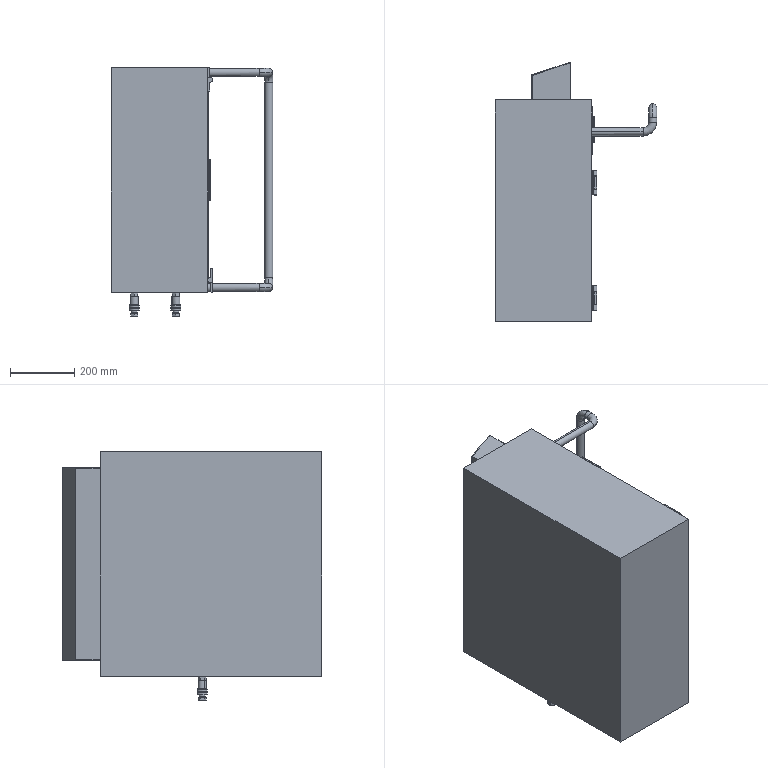Part | SolidWorks | features ReferencePattern 10, LocalLPattern 3, AEMSimFeature 1, MirrorCompFeat 1 | 26 solids | 1720 faces | box 502.5 x 808 x 775 mm | volume 40067990 mm3 | plane 1093 | cylinder 294 | spline 265 | cone 32 | torus 24 | sphere 12 | commonest cylinder face diameters 2 x44 5 x32 0.6 x26 8 x24 31 x21 6 x20